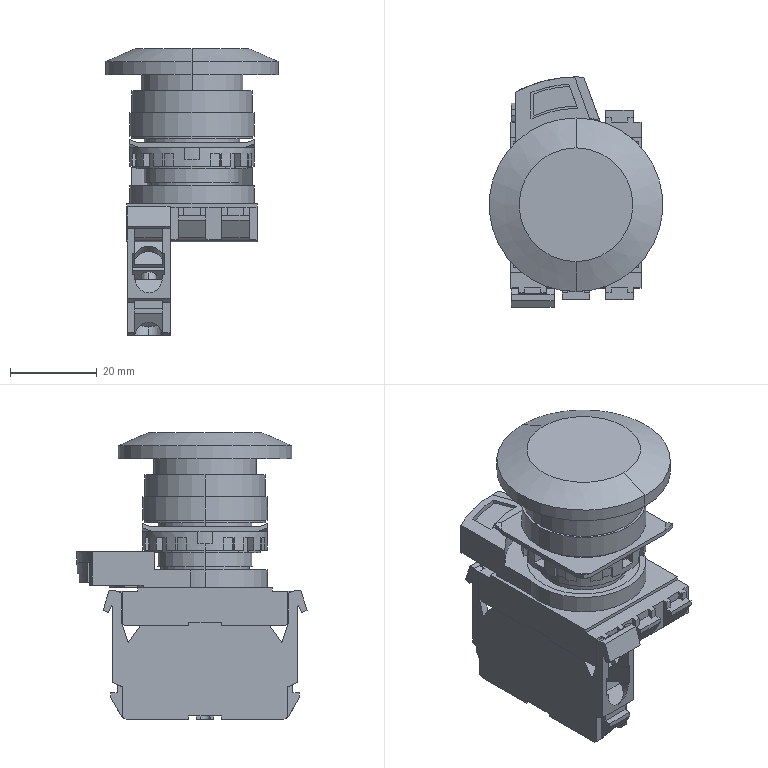Part | STEP file | A22NN_BMM_NGA_G100_NN | 5 solids | 516 faces | box 40 x 53 x 66 mm | volume 35883 mm3 | plane 406 | cylinder 108 | cone 2 | commonest cylinder face diameters 25.4 x10 27 x8 28.8 x7 4 x6 6.5 x6 20.8 x5